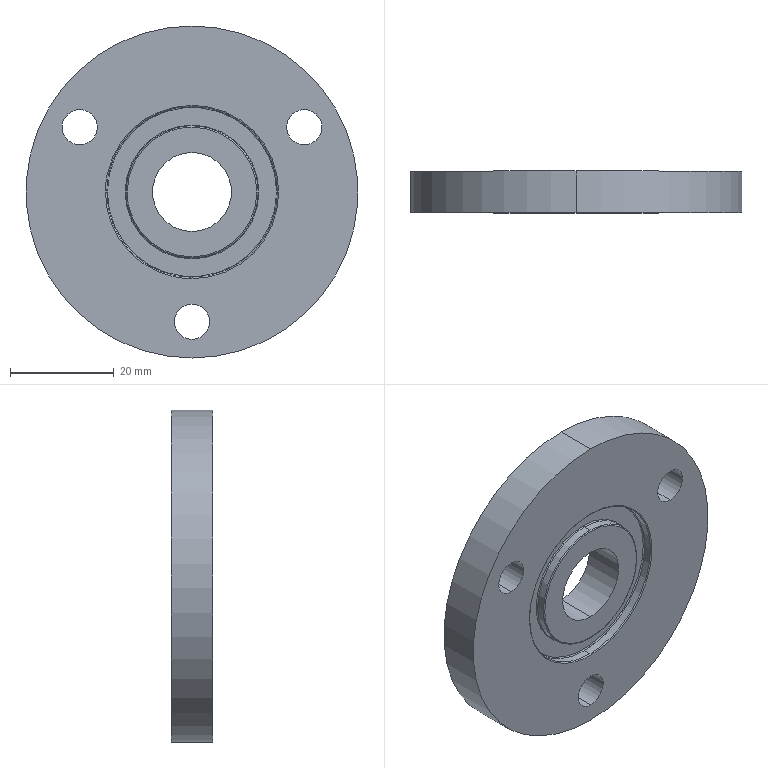Part | NX | features BREP 1 | 1 solid | 61 faces | box 64 x 8 x 64 mm | volume 20301 mm3 | torus 40 | cylinder 14 | plane 7 | commonest cylinder face diameters 6.8 x6 15.25 x2 25.4 x2 33 x2 64 x2